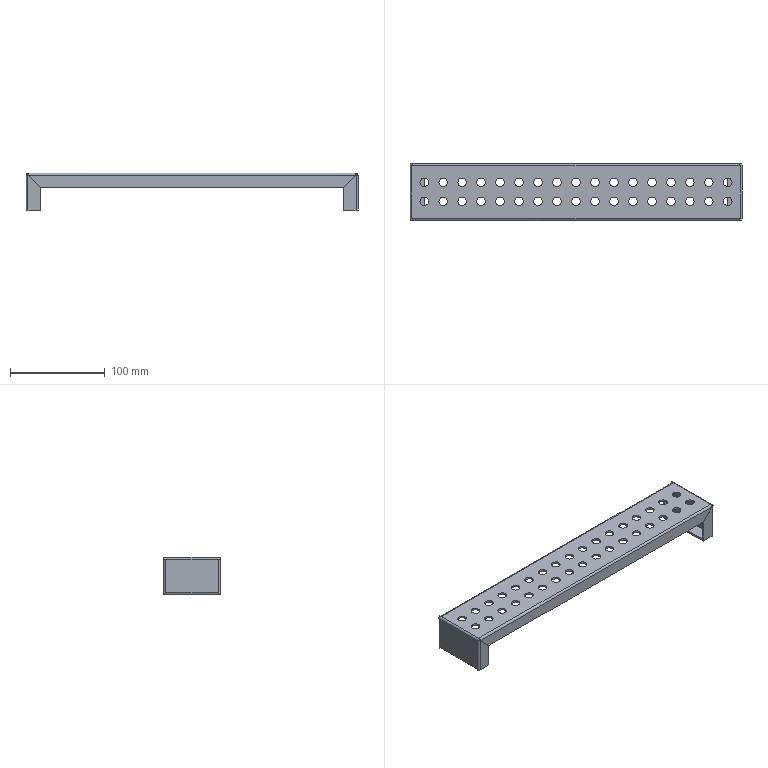Part | SolidWorks | features EdgeFlange 3, FlatPattern 1, ICE 1, SMBaseFlange 1, SheetMetal 1 | 1 solid | 166 faces | box 350 x 60 x 40 mm | volume 69257 mm3 | cylinder 88 | plane 70 | spline 8 | commonest cylinder face diameters 9 x68 0.2 x10 4.2 x10